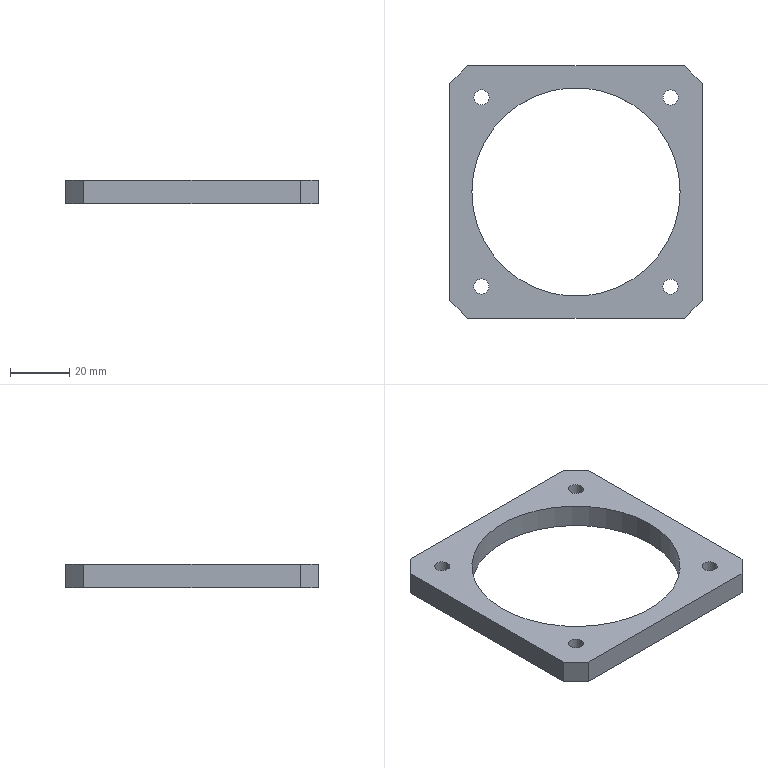NC program | NX | posted with a generic post | part box 85 x 85 x 8 mm
Lines 599 to 1875 of 1875:
(PLANAR_MILL_3 , TOOL : D10C-25L-35L)
N1124 T02 M6
N1126 G54
N1128 G17 G0 G90 X12.135 Y27.325 S4500 M3
N1130 G43 Z20. H2
N1132 Z3.
N1134 G94 G1 X11.608 Y27.587 Z2.995 F1500.
N1136 X8.07 Y28.822 Z2.962
N1138 X4.404 Y29.604 Z2.929
N1140 X0.67 Y29.923 Z2.897
N1142 X-3.075 Y29.772 Z2.864
N1144 X-6.771 Y29.154 Z2.831
N1146 X-10.362 Y28.079 Z2.799
N1148 X-13.79 Y26.564 Z2.766
N1150 X-16.11 Y25.224 Z2.743
N1152 X-19.007 Y23.12 Z2.711
N1154 X-21.632 Y20.685 Z2.68
N1156 X-23.948 Y17.953 Z2.649
N1158 X-25.92 Y14.965 Z2.618
N1160 X-27.522 Y11.763 Z2.586
N1162 X-28.729 Y8.392 Z2.555
N1164 X-29.526 Y4.901 Z2.524
N1166 X-29.9 Y1.34 Z2.493
N1168 Y-1.34 Z2.469
N1170 X-29.526 Y-4.901 Z2.438
N1172 X-28.729 Y-8.392 Z2.407
N1174 X-27.522 Y-11.763 Z2.375
N1176 X-25.92 Y-14.965 Z2.344
N1178 X-23.948 Y-17.953 Z2.313
N1180 X-21.632 Y-20.685 Z2.282
N1182 X-19.007 Y-23.12 Z2.25
N1184 X-16.11 Y-25.224 Z2.219
N1186 X-13.79 Y-26.564 Z2.196
N1188 X-10.362 Y-28.079 Z2.163
N1190 X-6.771 Y-29.154 Z2.13
N1192 X-3.075 Y-29.772 Z2.098
N1194 X0.67 Y-29.923 Z2.065
N1196 X4.404 Y-29.604 Z2.032
N1198 X8.07 Y-28.822 Z2.
N1200 X11.608 Y-27.587 Z1.967
N1202 X14.965 Y-25.92 Z1.934
N1204 X18.087 Y-23.847 Z1.901
N1206 X20.925 Y-21.399 Z1.869
N1208 X23.436 Y-18.616 Z1.836
N1210 X25.579 Y-15.542 Z1.803
N1212 X27.32 Y-12.223 Z1.771
N1214 X28.634 Y-8.713 Z1.738
N1216 X29.498 Y-5.066 Z1.705
N1218 X29.9 Y-1.34 Z1.672
N1220 Y1.34 Z1.649
N1222 X29.498 Y5.066 Z1.616
N1224 X28.634 Y8.713 Z1.584
N1226 X27.32 Y12.223 Z1.551
N1228 X25.579 Y15.542 Z1.518
N1230 X23.436 Y18.616 Z1.486
N1232 X20.925 Y21.399 Z1.453
N1234 X18.087 Y23.847 Z1.42
N1236 X14.965 Y25.92 Z1.387
N1238 X11.608 Y27.587 Z1.355
N1240 X8.07 Y28.822 Z1.322
N1242 X4.404 Y29.604 Z1.289
N1244 X0.67 Y29.923 Z1.257
N1246 X-3.075 Y29.772 Z1.224
N1248 X-6.771 Y29.154 Z1.191
N1250 X-10.362 Y28.079 Z1.159
N1252 X-13.79 Y26.564 Z1.126
N1254 X-16.11 Y25.224 Z1.102
N1256 X-19.007 Y23.12 Z1.071
N1258 X-21.632 Y20.685 Z1.04
N1260 X-23.948 Y17.953 Z1.009
N1262 X-25.92 Y14.965 Z0.977
N1264 X-27.522 Y11.763 Z0.946
N1266 X-28.729 Y8.392 Z0.915
N1268 X-29.526 Y4.901 Z0.884
N1270 X-29.9 Y1.34 Z0.852
N1272 Y-1.34 Z0.829
N1274 X-29.526 Y-4.901 Z0.798
N1276 X-28.729 Y-8.392 Z0.767
N1278 X-27.522 Y-11.763 Z0.735
N1280 X-25.92 Y-14.965 Z0.704
N1282 X-23.948 Y-17.953 Z0.673
N1284 X-21.632 Y-20.685 Z0.642
N1286 X-19.007 Y-23.12 Z0.61
N1288 X-16.11 Y-25.224 Z0.579
N1290 X-13.79 Y-26.564 Z0.556
N1292 X-10.362 Y-28.079 Z0.523
N1294 X-6.771 Y-29.154 Z0.49
N1296 X-3.075 Y-29.772 Z0.458
N1298 X0.67 Y-29.923 Z0.425
N1300 X4.404 Y-29.604 Z0.392
N1302 X8.07 Y-28.822 Z0.359
N1304 X11.608 Y-27.587 Z0.327
N1306 X14.965 Y-25.92 Z0.294
N1308 X18.087 Y-23.847 Z0.261
N1310 X20.925 Y-21.399 Z0.229
N1312 X23.436 Y-18.616 Z0.196
N1314 X25.579 Y-15.542 Z0.163
N1316 X27.32 Y-12.223 Z0.13
N1318 X28.634 Y-8.713 Z0.098
N1320 X29.498 Y-5.066 Z0.065
N1322 X29.9 Y-1.34 Z0.032
N1324 Y1.34 Z0.009
N1326 X29.498 Y5.066 Z-0.024
N1328 X28.634 Y8.713 Z-0.056
N1330 X27.32 Y12.223 Z-0.089
N1332 X25.579 Y15.542 Z-0.122
N1334 X23.436 Y18.616 Z-0.155
N1336 X20.925 Y21.399 Z-0.187
N1338 X18.087 Y23.847 Z-0.22
N1340 X14.965 Y25.92 Z-0.253
N1342 X11.608 Y27.587 Z-0.285
N1344 X8.07 Y28.822 Z-0.318
N1346 X4.404 Y29.604 Z-0.351
N1348 X0.67 Y29.923 Z-0.384
N1350 X-3.075 Y29.772 Z-0.416
N1352 X-6.771 Y29.154 Z-0.449
N1354 X-10.362 Y28.079 Z-0.482
N1356 X-13.79 Y26.564 Z-0.514
N1358 X-16.11 Y25.224 Z-0.538
N1360 X-19.007 Y23.12 Z-0.569
N1362 X-21.632 Y20.685 Z-0.6
N1364 X-23.948 Y17.953 Z-0.631
N1366 X-25.92 Y14.965 Z-0.663
N1368 X-27.522 Y11.763 Z-0.694
N1370 X-28.729 Y8.392 Z-0.725
N1372 X-29.526 Y4.901 Z-0.756
N1374 X-29.9 Y1.34 Z-0.788
N1376 Y-1.34 Z-0.811
N1378 X-29.526 Y-4.901 Z-0.842
N1380 X-28.729 Y-8.392 Z-0.874
N1382 X-27.522 Y-11.763 Z-0.905
N1384 X-25.92 Y-14.965 Z-0.936
N1386 X-23.948 Y-17.953 Z-0.967
N1388 X-21.632 Y-20.685 Z-0.999
N1390 X-19.007 Y-23.12 Z-1.03
N1392 X-16.11 Y-25.224 Z-1.061
N1394 X-13.79 Y-26.564 Z-1.084
N1396 X-10.362 Y-28.079 Z-1.117
N1398 X-6.771 Y-29.154 Z-1.15
N1400 X-3.075 Y-29.772 Z-1.183
N1402 X0.67 Y-29.923 Z-1.215
N1404 X4.404 Y-29.604 Z-1.248
N1406 X8.07 Y-28.822 Z-1.281
N1408 X11.608 Y-27.587 Z-1.313
N1410 X14.965 Y-25.92 Z-1.346
N1412 X18.087 Y-23.847 Z-1.379
N1414 X20.925 Y-21.399 Z-1.412
N1416 X23.436 Y-18.616 Z-1.444
N1418 X25.579 Y-15.542 Z-1.477
N1420 X27.32 Y-12.223 Z-1.51
N1422 X28.634 Y-8.713 Z-1.542
N1424 X29.498 Y-5.066 Z-1.575
N1426 X29.9 Y-1.34 Z-1.608
N1428 Y1.34 Z-1.631
N1430 X29.498 Y5.066 Z-1.664
N1432 X28.634 Y8.713 Z-1.697
N1434 X27.32 Y12.223 Z-1.729
N1436 X25.579 Y15.542 Z-1.762
N1438 X23.436 Y18.616 Z-1.795
N1440 X20.925 Y21.399 Z-1.827
N1442 X18.087 Y23.847 Z-1.86
N1444 X14.965 Y25.92 Z-1.893
N1446 X11.608 Y27.587 Z-1.926
N1448 X8.07 Y28.822 Z-1.958
N1450 X4.404 Y29.604 Z-1.991
N1452 X0.67 Y29.923 Z-2.024
N1454 X-3.075 Y29.772 Z-2.056
N1456 X-6.771 Y29.154 Z-2.089
N1458 X-10.362 Y28.079 Z-2.122
N1460 X-13.79 Y26.564 Z-2.154
N1462 X-16.11 Y25.224 Z-2.178
N1464 X-19.007 Y23.12 Z-2.209
N1466 X-21.632 Y20.685 Z-2.24
N1468 X-23.948 Y17.953 Z-2.272
N1470 X-25.92 Y14.965 Z-2.303
N1472 X-27.522 Y11.763 Z-2.334
N1474 X-28.729 Y8.392 Z-2.365
N1476 X-29.526 Y4.901 Z-2.397
N1478 X-29.9 Y1.34 Z-2.428
N1480 Y-1.34 Z-2.451
N1482 X-29.526 Y-4.901 Z-2.482
N1484 X-28.729 Y-8.392 Z-2.514
N1486 X-27.522 Y-11.763 Z-2.545
N1488 X-25.92 Y-14.965 Z-2.576
N1490 X-23.948 Y-17.953 Z-2.607
N1492 X-21.632 Y-20.685 Z-2.639
N1494 X-19.007 Y-23.12 Z-2.67
N1496 X-16.11 Y-25.224 Z-2.701
N1498 X-13.79 Y-26.564 Z-2.725
N1500 X-10.362 Y-28.079 Z-2.757
N1502 X-6.771 Y-29.154 Z-2.79
N1504 X-3.075 Y-29.772 Z-2.823
N1506 X0.67 Y-29.923 Z-2.855
N1508 X4.404 Y-29.604 Z-2.888
N1510 X8.07 Y-28.822 Z-2.921
N1512 X11.608 Y-27.587 Z-2.954
N1514 X14.965 Y-25.92 Z-2.986
N1516 X18.087 Y-23.847 Z-3.019
N1518 X20.925 Y-21.399 Z-3.052
N1520 X23.436 Y-18.616 Z-3.084
N1522 X25.579 Y-15.542 Z-3.117
N1524 X27.32 Y-12.223 Z-3.15
N1526 X28.634 Y-8.713 Z-3.182
N1528 X29.498 Y-5.066 Z-3.215
N1530 X29.9 Y-1.34 Z-3.248
N1532 Y1.34 Z-3.271
N1534 X29.498 Y5.066 Z-3.304
N1536 X28.634 Y8.713 Z-3.337
N1538 X27.32 Y12.223 Z-3.369
N1540 X25.579 Y15.542 Z-3.402
N1542 X23.436 Y18.616 Z-3.435
N1544 X20.925 Y21.399 Z-3.468
N1546 X18.087 Y23.847 Z-3.5
N1548 X14.965 Y25.92 Z-3.533
N1550 X11.608 Y27.587 Z-3.566
N1552 X8.07 Y28.822 Z-3.598
N1554 X4.404 Y29.604 Z-3.631
N1556 X0.67 Y29.923 Z-3.664
N1558 X-3.075 Y29.772 Z-3.696
N1560 X-6.771 Y29.154 Z-3.729
N1562 X-10.362 Y28.079 Z-3.762
N1564 X-13.79 Y26.564 Z-3.795
N1566 X-16.11 Y25.224 Z-3.818
N1568 X-19.007 Y23.12 Z-3.849
N1570 X-21.632 Y20.685 Z-3.88
N1572 X-23.948 Y17.953 Z-3.912
N1574 X-25.92 Y14.965 Z-3.943
N1576 X-27.522 Y11.763 Z-3.974
N1578 X-28.729 Y8.392 Z-4.005
N1580 X-29.526 Y4.901 Z-4.037
N1582 X-29.9 Y1.34 Z-4.068
N1584 Y-1.34 Z-4.091
N1586 X-29.526 Y-4.901 Z-4.123
N1588 X-28.729 Y-8.392 Z-4.154
N1590 X-27.522 Y-11.763 Z-4.185
N1592 X-25.92 Y-14.965 Z-4.216
N1594 X-23.948 Y-17.953 Z-4.248
N1596 X-21.632 Y-20.685 Z-4.279
N1598 X-19.007 Y-23.12 Z-4.31
N1600 X-16.11 Y-25.224 Z-4.341
N1602 X-13.79 Y-26.564 Z-4.365
N1604 X-10.362 Y-28.079 Z-4.397
N1606 X-6.771 Y-29.154 Z-4.43
N1608 X-3.075 Y-29.772 Z-4.463
N1610 X0.67 Y-29.923 Z-4.496
N1612 X4.404 Y-29.604 Z-4.528
N1614 X8.07 Y-28.822 Z-4.561
N1616 X11.608 Y-27.587 Z-4.594
N1618 X14.965 Y-25.92 Z-4.626
N1620 X18.087 Y-23.847 Z-4.659
N1622 X20.925 Y-21.399 Z-4.692
N1624 X23.436 Y-18.616 Z-4.724
N1626 X25.579 Y-15.542 Z-4.757
N1628 X27.32 Y-12.223 Z-4.79
N1630 X28.634 Y-8.713 Z-4.823
N1632 X29.498 Y-5.066 Z-4.855
N1634 X29.9 Y-1.34 Z-4.888
N1636 Y1.34 Z-4.911
N1638 X29.498 Y5.066 Z-4.944
N1640 X28.634 Y8.713 Z-4.977
N1642 X27.32 Y12.223 Z-5.01
N1644 X25.579 Y15.542 Z-5.042
N1646 X23.436 Y18.616 Z-5.075
N1648 X20.925 Y21.399 Z-5.108
N1650 X18.087 Y23.847 Z-5.14
N1652 X14.965 Y25.92 Z-5.173
N1654 X11.608 Y27.587 Z-5.206
N1656 X8.07 Y28.822 Z-5.238
N1658 X4.404 Y29.604 Z-5.271
N1660 X0.67 Y29.923 Z-5.304
N1662 X-3.075 Y29.772 Z-5.337
N1664 X-6.771 Y29.154 Z-5.369
N1666 X-10.362 Y28.079 Z-5.402
N1668 X-13.79 Y26.564 Z-5.435
N1670 X-16.11 Y25.224 Z-5.458
N1672 X-19.007 Y23.12 Z-5.489
N1674 X-21.632 Y20.685 Z-5.521
N1676 X-23.948 Y17.953 Z-5.552
N1678 X-25.92 Y14.965 Z-5.583
N1680 X-27.522 Y11.763 Z-5.614
N1682 X-28.729 Y8.392 Z-5.646
N1684 X-29.526 Y4.901 Z-5.677
N1686 X-29.9 Y1.34 Z-5.708
N1688 Y-1.34 Z-5.731
N1690 X-29.526 Y-4.901 Z-5.763
N1692 X-28.729 Y-8.392 Z-5.794
N1694 X-27.522 Y-11.763 Z-5.825
N1696 X-25.92 Y-14.965 Z-5.856
N1698 X-23.948 Y-17.953 Z-5.888
N1700 X-21.632 Y-20.685 Z-5.919
N1702 X-19.007 Y-23.12 Z-5.95
N1704 X-16.11 Y-25.224 Z-5.981
N1706 X-13.79 Y-26.564 Z-6.005
N1708 X-10.362 Y-28.079 Z-6.038
N1710 X-6.771 Y-29.154 Z-6.07
N1712 X-3.075 Y-29.772 Z-6.103
N1714 X0.67 Y-29.923 Z-6.136
N1716 X4.404 Y-29.604 Z-6.168
N1718 X8.07 Y-28.822 Z-6.201
N1720 X11.608 Y-27.587 Z-6.234
N1722 X14.965 Y-25.92 Z-6.266
N1724 X18.087 Y-23.847 Z-6.299
N1726 X20.925 Y-21.399 Z-6.332
N1728 X23.436 Y-18.616 Z-6.365
N1730 X25.579 Y-15.542 Z-6.397
N1732 X27.32 Y-12.223 Z-6.43
N1734 X28.634 Y-8.713 Z-6.463
N1736 X29.498 Y-5.066 Z-6.495
N1738 X29.9 Y-1.34 Z-6.528
N1740 Y1.34 Z-6.552
N1742 X29.498 Y5.066 Z-6.584
N1744 X28.634 Y8.713 Z-6.617
N1746 X27.32 Y12.223 Z-6.65
N1748 X25.579 Y15.542 Z-6.682
N1750 X23.436 Y18.616 Z-6.715
N1752 X20.925 Y21.399 Z-6.748
N1754 X18.087 Y23.847 Z-6.78
N1756 X14.965 Y25.92 Z-6.813
N1758 X11.608 Y27.587 Z-6.846
N1760 X8.07 Y28.822 Z-6.879
N1762 X4.404 Y29.604 Z-6.911
N1764 X0.67 Y29.923 Z-6.944
N1766 X-3.075 Y29.772 Z-6.977
N1768 X-6.771 Y29.154 Z-7.009
N1770 X-10.362 Y28.079 Z-7.042
N1772 X-13.79 Y26.564 Z-7.075
N1774 X-16.11 Y25.224 Z-7.098
N1776 X-19.007 Y23.12 Z-7.129
N1778 X-21.632 Y20.685 Z-7.161
N1780 X-23.948 Y17.953 Z-7.192
N1782 X-25.92 Y14.965 Z-7.223
N1784 X-27.522 Y11.763 Z-7.254
N1786 X-28.729 Y8.392 Z-7.286
N1788 X-29.526 Y4.901 Z-7.317
N1790 X-29.9 Y1.34 Z-7.348
N1792 Y-1.34 Z-7.372
N1794 X-29.526 Y-4.901 Z-7.403
N1796 X-28.729 Y-8.392 Z-7.434
N1798 X-27.522 Y-11.763 Z-7.465
N1800 X-25.92 Y-14.965 Z-7.497
N1802 X-23.948 Y-17.953 Z-7.528
N1804 X-21.632 Y-20.685 Z-7.559
N1806 X-19.007 Y-23.12 Z-7.59
N1808 X-16.11 Y-25.224 Z-7.622
N1810 X-13.79 Y-26.564 Z-7.645
N1812 X-10.362 Y-28.079 Z-7.678
N1814 X-6.771 Y-29.154 Z-7.71
N1816 X-3.075 Y-29.772 Z-7.743
N1818 X0.67 Y-29.923 Z-7.776
N1820 X4.404 Y-29.604 Z-7.808
N1822 X8.07 Y-28.822 Z-7.841
N1824 X11.608 Y-27.587 Z-7.874
N1826 X14.965 Y-25.92 Z-7.907
N1828 X18.087 Y-23.847 Z-7.939
N1830 X20.925 Y-21.399 Z-7.972
N1832 X23.436 Y-18.616 Z-8.005
N1834 X25.579 Y-15.542 Z-8.037
N1836 X27.32 Y-12.223 Z-8.07
N1838 X28.634 Y-8.713 Z-8.103
N1840 X29.498 Y-5.066 Z-8.136
N1842 X29.9 Y-1.34 Z-8.168
N1844 Y1.34 Z-8.192
N1846 X29.498 Y5.066 Z-8.224
N1848 X28.634 Y8.713 Z-8.257
N1850 X27.32 Y12.223 Z-8.29
N1852 X25.579 Y15.542 Z-8.322
N1854 X23.436 Y18.616 Z-8.355
N1856 X20.925 Y21.399 Z-8.388
N1858 X18.087 Y23.847 Z-8.421
N1860 X14.965 Y25.92 Z-8.453
N1862 X11.608 Y27.587 Z-8.486
N1864 X8.07 Y28.822 Z-8.519
N1866 X4.404 Y29.604 Z-8.551
N1868 X0.67 Y29.923 Z-8.584
N1870 X-3.075 Y29.772 Z-8.617
N1872 X-6.771 Y29.154 Z-8.65
N1874 X-10.362 Y28.079 Z-8.682
N1876 X-13.79 Y26.564 Z-8.715
N1878 X-16.11 Y25.224 Z-8.738
N1880 X-19.007 Y23.12 Z-8.77
N1882 X-21.632 Y20.685 Z-8.801
N1884 X-23.948 Y17.953 Z-8.832
N1886 X-25.92 Y14.965 Z-8.863
N1888 X-27.522 Y11.763 Z-8.895
N1890 X-28.729 Y8.392 Z-8.926
N1892 X-29.526 Y4.901 Z-8.957
N1894 X-29.9 Y1.34 Z-8.988
N1896 Y0. Z-9.
N1898 G3 X0. Y-29.9 R29.9
N1900 X-29.9 Y0. R-29.9
N1902 G1 Z-6.
N1904 G0 Z20.
(PLANAR_MILL_3_COPY_1 , TOOL : D10C-25L-35L)
N1906 X-5.416 Y-24.318
N1908 Z3.
N1910 G1 X-5.157 Y-24.391 Z2.998
N1912 X-1.875 Y-24.859 Z2.969
N1914 X1.44 Y-24.888 Z2.94
N1916 X4.73 Y-24.477 Z2.911
N1918 X7.936 Y-23.633 Z2.882
N1920 X11.002 Y-22.371 Z2.853
N1922 X13.873 Y-20.713 Z2.824
N1924 X16.499 Y-18.689 Z2.795
N1926 X18.833 Y-16.335 Z2.766
N1928 X20.834 Y-13.691 Z2.737
N1930 X22.466 Y-10.806 Z2.708
N1932 X23.702 Y-7.729 Z2.679
N1934 X24.518 Y-4.516 Z2.65
N1936 X24.9 Y-1.223 Z2.622
N1938 Y1.223 Z2.6
N1940 X24.518 Y4.516 Z2.571
N1942 X23.702 Y7.729 Z2.542
N1944 X22.466 Y10.806 Z2.513
N1946 X20.834 Y13.691 Z2.484
N1948 X18.833 Y16.335 Z2.456
N1950 X16.499 Y18.689 Z2.427
N1952 X13.873 Y20.713 Z2.398
N1954 X11.002 Y22.371 Z2.369
N1956 X7.936 Y23.633 Z2.34
N1958 X4.73 Y24.477 Z2.311
N1960 X1.44 Y24.888 Z2.282
N1962 X-1.875 Y24.859 Z2.253
N1964 X-5.157 Y24.391 Z2.224
N1966 X-8.348 Y23.491 Z2.195
N1968 X-11.391 Y22.175 Z2.166
N1970 X-13.509 Y20.953 Z2.145
N1972 X-16.217 Y18.934 Z2.115
N1974 X-18.627 Y16.569 Z2.086
N1976 X-20.696 Y13.899 Z2.056
N1978 X-22.385 Y10.974 Z2.027
N1980 X-23.663 Y7.848 Z1.997
N1982 X-24.506 Y4.577 Z1.968
N1984 X-24.9 Y1.223 Z1.939
N1986 Y-1.223 Z1.917
N1988 X-24.506 Y-4.577 Z1.888
N1990 X-23.663 Y-7.848 Z1.858
N1992 X-22.385 Y-10.974 Z1.829
N1994 X-20.696 Y-13.899 Z1.799
N1996 X-18.627 Y-16.569 Z1.77
N1998 X-16.217 Y-18.934 Z1.74
N2000 X-13.509 Y-20.953 Z1.711
N2002 X-11.391 Y-22.175 Z1.69
N2004 X-8.348 Y-23.491 Z1.661
N2006 X-5.157 Y-24.391 Z1.632
N2008 X-1.875 Y-24.859 Z1.603
N2010 X1.44 Y-24.888 Z1.574
N2012 X4.73 Y-24.477 Z1.545
N2014 X7.936 Y-23.633 Z1.516
N2016 X11.002 Y-22.371 Z1.487
N2018 X13.873 Y-20.713 Z1.458
N2020 X16.499 Y-18.689 Z1.429
N2022 X18.833 Y-16.335 Z1.4
N2024 X20.834 Y-13.691 Z1.371
N2026 X22.466 Y-10.806 Z1.342
N2028 X23.702 Y-7.729 Z1.313
N2030 X24.518 Y-4.516 Z1.284
N2032 X24.9 Y-1.223 Z1.256
N2034 Y1.223 Z1.234
N2036 X24.518 Y4.516 Z1.205
N2038 X23.702 Y7.729 Z1.176
N2040 X22.466 Y10.806 Z1.147
N2042 X20.834 Y13.691 Z1.118
N2044 X18.833 Y16.335 Z1.09
N2046 X16.499 Y18.689 Z1.061
N2048 X13.873 Y20.713 Z1.032
N2050 X11.002 Y22.371 Z1.003
N2052 X7.936 Y23.633 Z0.974
N2054 X4.73 Y24.477 Z0.945
N2056 X1.44 Y24.888 Z0.916
N2058 X-1.875 Y24.859 Z0.887
N2060 X-5.157 Y24.391 Z0.858
N2062 X-8.348 Y23.491 Z0.829
N2064 X-11.391 Y22.175 Z0.8
N2066 X-13.509 Y20.953 Z0.779
N2068 X-16.217 Y18.934 Z0.749
N2070 X-18.627 Y16.569 Z0.72
N2072 X-20.696 Y13.899 Z0.69
N2074 X-22.385 Y10.974 Z0.661
N2076 X-23.663 Y7.848 Z0.632
N2078 X-24.506 Y4.577 Z0.602
N2080 X-24.9 Y1.223 Z0.573
N2082 Y-1.223 Z0.551
N2084 X-24.506 Y-4.577 Z0.522
N2086 X-23.663 Y-7.848 Z0.492
N2088 X-22.385 Y-10.974 Z0.463
N2090 X-20.696 Y-13.899 Z0.433
N2092 X-18.627 Y-16.569 Z0.404
N2094 X-16.217 Y-18.934 Z0.374
N2096 X-13.509 Y-20.953 Z0.345
N2098 X-11.391 Y-22.175 Z0.324
N2100 X-8.348 Y-23.491 Z0.295
N2102 X-5.157 Y-24.391 Z0.266
N2104 X-1.875 Y-24.859 Z0.237
N2106 X1.44 Y-24.888 Z0.208
N2108 X4.73 Y-24.477 Z0.179
N2110 X7.936 Y-23.633 Z0.15
N2112 X11.002 Y-22.371 Z0.121
N2114 X13.873 Y-20.713 Z0.092
N2116 X16.499 Y-18.689 Z0.063
N2118 X18.833 Y-16.335 Z0.034
N2120 X20.834 Y-13.691 Z0.005
N2122 X22.466 Y-10.806 Z-0.024
N2124 X23.702 Y-7.729 Z-0.053
N2126 X24.518 Y-4.516 Z-0.082
N2128 X24.9 Y-1.223 Z-0.11
N2130 Y1.223 Z-0.132
N2132 X24.518 Y4.516 Z-0.161
N2134 X23.702 Y7.729 Z-0.19
N2136 X22.466 Y10.806 Z-0.219
N2138 X20.834 Y13.691 Z-0.248
N2140 X18.833 Y16.335 Z-0.276
N2142 X16.499 Y18.689 Z-0.305
N2144 X13.873 Y20.713 Z-0.334
N2146 X11.002 Y22.371 Z-0.363
N2148 X7.936 Y23.633 Z-0.392
N2150 X4.73 Y24.477 Z-0.421
N2152 X1.44 Y24.888 Z-0.45
N2154 X-1.875 Y24.859 Z-0.479
N2156 X-5.157 Y24.391 Z-0.508
N2158 X-8.348 Y23.491 Z-0.537
N2160 X-11.391 Y22.175 Z-0.566
N2162 X-13.509 Y20.953 Z-0.587
N2164 X-16.217 Y18.934 Z-0.617
N2166 X-18.627 Y16.569 Z-0.646
N2168 X-20.696 Y13.899 Z-0.676
N2170 X-22.385 Y10.974 Z-0.705
N2172 X-23.663 Y7.848 Z-0.734
N2174 X-24.506 Y4.577 Z-0.764
N2176 X-24.9 Y1.223 Z-0.793
N2178 Y-1.223 Z-0.815
N2180 X-24.506 Y-4.577 Z-0.844
N2182 X-23.663 Y-7.848 Z-0.874
N2184 X-22.385 Y-10.974 Z-0.903
N2186 X-20.696 Y-13.899 Z-0.933
N2188 X-18.627 Y-16.569 Z-0.962
N2190 X-16.217 Y-18.934 Z-0.992
N2192 X-13.509 Y-20.953 Z-1.021
N2194 X-11.391 Y-22.175 Z-1.042
N2196 X-8.348 Y-23.491 Z-1.071
N2198 X-5.157 Y-24.391 Z-1.1
N2200 X-1.875 Y-24.859 Z-1.129
N2202 X1.44 Y-24.888 Z-1.158
N2204 X4.73 Y-24.477 Z-1.187
N2206 X7.936 Y-23.633 Z-1.216
N2208 X11.002 Y-22.371 Z-1.245
N2210 X13.873 Y-20.713 Z-1.274
N2212 X16.499 Y-18.689 Z-1.303
N2214 X18.833 Y-16.335 Z-1.332
N2216 X20.834 Y-13.691 Z-1.361
N2218 X22.466 Y-10.806 Z-1.39
N2220 X23.702 Y-7.729 Z-1.419
N2222 X24.518 Y-4.516 Z-1.447
N2224 X24.9 Y-1.223 Z-1.476
N2226 Y1.223 Z-1.498
N2228 X24.518 Y4.516 Z-1.527
N2230 X23.702 Y7.729 Z-1.556
N2232 X22.466 Y10.806 Z-1.585
N2234 X20.834 Y13.691 Z-1.613
N2236 X18.833 Y16.335 Z-1.642
N2238 X16.499 Y18.689 Z-1.671
N2240 X13.873 Y20.713 Z-1.7
N2242 X11.002 Y22.371 Z-1.729
N2244 X7.936 Y23.633 Z-1.758
N2246 X4.73 Y24.477 Z-1.787
N2248 X1.44 Y24.888 Z-1.816
N2250 X-1.875 Y24.859 Z-1.845
N2252 X-5.157 Y24.391 Z-1.874
N2254 X-8.348 Y23.491 Z-1.903
N2256 X-11.391 Y22.175 Z-1.932
N2258 X-13.509 Y20.953 Z-1.953
N2260 X-16.217 Y18.934 Z-1.983
N2262 X-18.627 Y16.569 Z-2.012
N2264 X-20.696 Y13.899 Z-2.042
N2266 X-22.385 Y10.974 Z-2.071
N2268 X-23.663 Y7.848 Z-2.1
N2270 X-24.506 Y4.577 Z-2.13
N2272 X-24.9 Y1.223 Z-2.159
N2274 Y-1.223 Z-2.181
N2276 X-24.506 Y-4.577 Z-2.21
N2278 X-23.663 Y-7.848 Z-2.24
N2280 X-22.385 Y-10.974 Z-2.269
N2282 X-20.696 Y-13.899 Z-2.299
N2284 X-18.627 Y-16.569 Z-2.328
N2286 X-16.217 Y-18.934 Z-2.358
N2288 X-13.509 Y-20.953 Z-2.387
N2290 X-11.391 Y-22.175 Z-2.408
N2292 X-8.348 Y-23.491 Z-2.437
N2294 X-5.157 Y-24.391 Z-2.466
N2296 X-1.875 Y-24.859 Z-2.495
N2298 X1.44 Y-24.888 Z-2.524
N2300 X4.73 Y-24.477 Z-2.553
N2302 X7.936 Y-23.633 Z-2.582
N2304 X11.002 Y-22.371 Z-2.611
N2306 X13.873 Y-20.713 Z-2.64
N2308 X16.499 Y-18.689 Z-2.669
N2310 X18.833 Y-16.335 Z-2.698
N2312 X20.834 Y-13.691 Z-2.727
N2314 X22.466 Y-10.806 Z-2.756
N2316 X23.702 Y-7.729 Z-2.785
N2318 X24.518 Y-4.516 Z-2.813
N2320 X24.9 Y-1.223 Z-2.842
N2322 Y1.223 Z-2.864
N2324 X24.518 Y4.516 Z-2.893
N2326 X23.702 Y7.729 Z-2.922
N2328 X22.466 Y10.806 Z-2.951
N2330 X20.834 Y13.691 Z-2.979
N2332 X18.833 Y16.335 Z-3.008
N2334 X16.499 Y18.689 Z-3.037
N2336 X13.873 Y20.713 Z-3.066
N2338 X11.002 Y22.371 Z-3.095
N2340 X7.936 Y23.633 Z-3.124
N2342 X4.73 Y24.477 Z-3.153
N2344 X1.44 Y24.888 Z-3.182
N2346 X-1.875 Y24.859 Z-3.211
N2348 X-5.157 Y24.391 Z-3.24
N2350 X-8.348 Y23.491 Z-3.269
N2352 X-11.391 Y22.175 Z-3.298
N2354 X-13.509 Y20.953 Z-3.319
N2356 X-16.217 Y18.934 Z-3.349
N2358 X-18.627 Y16.569 Z-3.378
N2360 X-20.696 Y13.899 Z-3.407
N2362 X-22.385 Y10.974 Z-3.437
N2364 X-23.663 Y7.848 Z-3.466
N2366 X-24.506 Y4.577 Z-3.496
N2368 X-24.9 Y1.223 Z-3.525
N2370 Y-1.223 Z-3.547
N2372 X-24.506 Y-4.577 Z-3.576
N2374 X-23.663 Y-7.848 Z-3.606
N2376 X-22.385 Y-10.974 Z-3.635
N2378 X-20.696 Y-13.899 Z-3.665
N2380 X-18.627 Y-16.569 Z-3.694
N2382 X-16.217 Y-18.934 Z-3.724
N2384 X-13.509 Y-20.953 Z-3.753
N2386 X-11.391 Y-22.175 Z-3.774
N2388 X-8.348 Y-23.491 Z-3.803
N2390 X-5.157 Y-24.391 Z-3.832
N2392 X-1.875 Y-24.859 Z-3.861
N2394 X1.44 Y-24.888 Z-3.89
N2396 X4.73 Y-24.477 Z-3.919
N2398 X7.936 Y-23.633 Z-3.948
N2400 X11.002 Y-22.371 Z-3.977
N2402 X13.873 Y-20.713 Z-4.006
N2404 X16.499 Y-18.689 Z-4.035
N2406 X18.833 Y-16.335 Z-4.064
N2408 X20.834 Y-13.691 Z-4.093
N2410 X22.466 Y-10.806 Z-4.122
N2412 X23.702 Y-7.729 Z-4.151
N2414 X24.518 Y-4.516 Z-4.179
N2416 X24.9 Y-1.223 Z-4.208
N2418 Y1.223 Z-4.23
N2420 X24.518 Y4.516 Z-4.259
N2422 X23.702 Y7.729 Z-4.288
N2424 X22.466 Y10.806 Z-4.317
N2426 X20.834 Y13.691 Z-4.345
N2428 X18.833 Y16.335 Z-4.374
N2430 X16.499 Y18.689 Z-4.403
N2432 X13.873 Y20.713 Z-4.432
N2434 X11.002 Y22.371 Z-4.461
N2436 X7.936 Y23.633 Z-4.49
N2438 X4.73 Y24.477 Z-4.519
N2440 X1.44 Y24.888 Z-4.548
N2442 X-1.875 Y24.859 Z-4.577
N2444 X-5.157 Y24.391 Z-4.606
N2446 X-8.348 Y23.491 Z-4.635
N2448 X-11.391 Y22.175 Z-4.664
N2450 X-13.509 Y20.953 Z-4.685
N2452 X-16.217 Y18.934 Z-4.715
N2454 X-18.627 Y16.569 Z-4.744
N2456 X-20.696 Y13.899 Z-4.773
N2458 X-22.385 Y10.974 Z-4.803
N2460 X-23.663 Y7.848 Z-4.832
N2462 X-24.506 Y4.577 Z-4.862
N2464 X-24.9 Y1.223 Z-4.891
N2466 Y-1.223 Z-4.913
N2468 X-24.506 Y-4.577 Z-4.942
N2470 X-23.663 Y-7.848 Z-4.972
N2472 X-22.385 Y-10.974 Z-5.001
N2474 X-20.696 Y-13.899 Z-5.031
N2476 X-18.627 Y-16.569 Z-5.06
N2478 X-16.217 Y-18.934 Z-5.09
N2480 X-13.509 Y-20.953 Z-5.119
N2482 X-11.391 Y-22.175 Z-5.14
N2484 X-8.348 Y-23.491 Z-5.169
N2486 X-5.157 Y-24.391 Z-5.198
N2488 X-1.875 Y-24.859 Z-5.227
N2490 X1.44 Y-24.888 Z-5.256
N2492 X4.73 Y-24.477 Z-5.285
N2494 X7.936 Y-23.633 Z-5.314
N2496 X11.002 Y-22.371 Z-5.343
N2498 X13.873 Y-20.713 Z-5.372
N2500 X16.499 Y-18.689 Z-5.401
N2502 X18.833 Y-16.335 Z-5.43
N2504 X20.834 Y-13.691 Z-5.459
N2506 X22.466 Y-10.806 Z-5.488
N2508 X23.702 Y-7.729 Z-5.517
N2510 X24.518 Y-4.516 Z-5.545
N2512 X24.9 Y-1.223 Z-5.574
N2514 Y1.223 Z-5.596
N2516 X24.518 Y4.516 Z-5.625
N2518 X23.702 Y7.729 Z-5.654
N2520 X22.466 Y10.806 Z-5.683
N2522 X20.834 Y13.691 Z-5.711
N2524 X18.833 Y16.335 Z-5.74
N2526 X16.499 Y18.689 Z-5.769
N2528 X13.873 Y20.713 Z-5.798
N2530 X11.002 Y22.371 Z-5.827
N2532 X7.936 Y23.633 Z-5.856
N2534 X4.73 Y24.477 Z-5.885
N2536 X1.44 Y24.888 Z-5.914
N2538 X-1.875 Y24.859 Z-5.943
N2540 X-5.157 Y24.391 Z-5.972
N2542 X-8.348 Y23.491 Z-6.001
N2544 X-11.391 Y22.175 Z-6.03
N2546 X-13.509 Y20.953 Z-6.051
N2548 X-16.217 Y18.934 Z-6.081
N2550 X-18.627 Y16.569 Z-6.11
N2552 X-20.696 Y13.899 Z-6.139
N2554 X-22.385 Y10.974 Z-6.169
N2556 X-23.663 Y7.848 Z-6.198
N2558 X-24.506 Y4.577 Z-6.228
N2560 X-24.9 Y1.223 Z-6.257
N2562 Y-1.223 Z-6.279
N2564 X-24.506 Y-4.577 Z-6.308
N2566 X-23.663 Y-7.848 Z-6.338
N2568 X-22.385 Y-10.974 Z-6.367
N2570 X-20.696 Y-13.899 Z-6.397
N2572 X-18.627 Y-16.569 Z-6.426
N2574 X-16.217 Y-18.934 Z-6.456
N2576 X-13.509 Y-20.953 Z-6.485
N2578 X-11.391 Y-22.175 Z-6.506
N2580 X-8.348 Y-23.491 Z-6.535
N2582 X-5.157 Y-24.391 Z-6.564
N2584 X-1.875 Y-24.859 Z-6.593
N2586 X1.44 Y-24.888 Z-6.622
N2588 X4.73 Y-24.477 Z-6.651
N2590 X7.936 Y-23.633 Z-6.68
N2592 X11.002 Y-22.371 Z-6.709
N2594 X13.873 Y-20.713 Z-6.738
N2596 X16.499 Y-18.689 Z-6.767
N2598 X18.833 Y-16.335 Z-6.796
N2600 X20.834 Y-13.691 Z-6.825
N2602 X22.466 Y-10.806 Z-6.854
N2604 X23.702 Y-7.729 Z-6.882
N2606 X24.518 Y-4.516 Z-6.911
N2608 X24.9 Y-1.223 Z-6.94
N2610 Y1.223 Z-6.962
N2612 X24.518 Y4.516 Z-6.991
N2614 X23.702 Y7.729 Z-7.02
N2616 X22.466 Y10.806 Z-7.048
N2618 X20.834 Y13.691 Z-7.077
N2620 X18.833 Y16.335 Z-7.106
N2622 X16.499 Y18.689 Z-7.135
N2624 X13.873 Y20.713 Z-7.164
N2626 X11.002 Y22.371 Z-7.193
N2628 X7.936 Y23.633 Z-7.222
N2630 X4.73 Y24.477 Z-7.251
N2632 X1.44 Y24.888 Z-7.28
N2634 X-1.875 Y24.859 Z-7.309
N2636 X-5.157 Y24.391 Z-7.338
N2638 X-8.348 Y23.491 Z-7.367
N2640 X-11.391 Y22.175 Z-7.396
N2642 X-13.509 Y20.953 Z-7.417
N2644 X-16.217 Y18.934 Z-7.446
N2646 X-18.627 Y16.569 Z-7.476
N2648 X-20.696 Y13.899 Z-7.505
N2650 X-22.385 Y10.974 Z-7.535
N2652 X-23.663 Y7.848 Z-7.564
N2654 X-24.506 Y4.577 Z-7.594
N2656 X-24.9 Y1.223 Z-7.623
N2658 Y-1.223 Z-7.645
N2660 X-24.506 Y-4.577 Z-7.674
N2662 X-23.663 Y-7.848 Z-7.704
N2664 X-22.385 Y-10.974 Z-7.733
N2666 X-20.696 Y-13.899 Z-7.763
N2668 X-18.627 Y-16.569 Z-7.792
N2670 X-16.217 Y-18.934 Z-7.822
N2672 X-13.509 Y-20.953 Z-7.851
N2674 X-11.391 Y-22.175 Z-7.872
N2676 X-8.348 Y-23.491 Z-7.901
N2678 X-5.157 Y-24.391 Z-7.93
N2680 X-1.875 Y-24.859 Z-7.959
N2682 X1.44 Y-24.888 Z-7.988
N2684 X4.73 Y-24.477 Z-8.017
N2686 X7.936 Y-23.633 Z-8.046
N2688 X11.002 Y-22.371 Z-8.075
N2690 X13.873 Y-20.713 Z-8.104
N2692 X16.499 Y-18.689 Z-8.133
N2694 X18.833 Y-16.335 Z-8.162
N2696 X20.834 Y-13.691 Z-8.191
N2698 X22.466 Y-10.806 Z-8.22
N2700 X23.702 Y-7.729 Z-8.248
N2702 X24.518 Y-4.516 Z-8.277
N2704 X24.9 Y-1.223 Z-8.306
N2706 Y1.223 Z-8.328
N2708 X24.518 Y4.516 Z-8.357
N2710 X23.702 Y7.729 Z-8.386
N2712 X22.466 Y10.806 Z-8.414
N2714 X20.834 Y13.691 Z-8.443
N2716 X18.833 Y16.335 Z-8.472
N2718 X16.499 Y18.689 Z-8.501
N2720 X13.873 Y20.713 Z-8.53
N2722 X11.002 Y22.371 Z-8.559
N2724 X7.936 Y23.633 Z-8.588
N2726 X4.73 Y24.477 Z-8.617
N2728 X1.44 Y24.888 Z-8.646
N2730 X-1.875 Y24.859 Z-8.675
N2732 X-5.157 Y24.391 Z-8.704
N2734 X-8.348 Y23.491 Z-8.733
N2736 X-11.391 Y22.175 Z-8.762
N2738 X-13.509 Y20.953 Z-8.783
N2740 X-16.217 Y18.934 Z-8.812
N2742 X-18.627 Y16.569 Z-8.842
N2744 X-20.696 Y13.899 Z-8.871
N2746 X-22.385 Y10.974 Z-8.901
N2748 X-23.663 Y7.848 Z-8.93
N2750 X-24.506 Y4.577 Z-8.96
N2752 X-24.9 Y1.223 Z-8.989
N2754 Y0. Z-9.
N2756 G3 X0. Y-24.9 R24.9
N2758 X-24.9 Y0. R-24.9
N2760 G1 Z-6.
N2762 G0 Z20.
N2764 X12.135 Y27.325
N2766 Z3.
N2768 G1 X11.608 Y27.587 Z2.995
N2770 X8.07 Y28.822 Z2.962
N2772 X4.404 Y29.604 Z2.929
N2774 X0.67 Y29.923 Z2.897
N2776 X-3.075 Y29.772 Z2.864
N2778 X-6.771 Y29.154 Z2.831
N2780 X-10.362 Y28.079 Z2.799
N2782 X-13.79 Y26.564 Z2.766
N2784 X-16.11 Y25.224 Z2.743
N2786 X-19.007 Y23.12 Z2.711
N2788 X-21.632 Y20.685 Z2.68
N2790 X-23.948 Y17.953 Z2.649
N2792 X-25.92 Y14.965 Z2.618
N2794 X-27.522 Y11.763 Z2.586
N2796 X-28.729 Y8.392 Z2.555
N2798 X-29.526 Y4.901 Z2.524
N2800 X-29.9 Y1.34 Z2.493
N2802 Y-1.34 Z2.469
N2804 X-29.526 Y-4.901 Z2.438
N2806 X-28.729 Y-8.392 Z2.407
N2808 X-27.522 Y-11.763 Z2.375
N2810 X-25.92 Y-14.965 Z2.344
N2812 X-23.948 Y-17.953 Z2.313
N2814 X-21.632 Y-20.685 Z2.282
N2816 X-19.007 Y-23.12 Z2.25
N2818 X-16.11 Y-25.224 Z2.219
N2820 X-13.79 Y-26.564 Z2.196
N2822 X-10.362 Y-28.079 Z2.163
N2824 X-6.771 Y-29.154 Z2.13
N2826 X-3.075 Y-29.772 Z2.098
N2828 X0.67 Y-29.923 Z2.065
N2830 X4.404 Y-29.604 Z2.032
N2832 X8.07 Y-28.822 Z2.
N2834 X11.608 Y-27.587 Z1.967
N2836 X14.965 Y-25.92 Z1.934
N2838 X18.087 Y-23.847 Z1.901
N2840 X20.925 Y-21.399 Z1.869
N2842 X23.436 Y-18.616 Z1.836
N2844 X25.579 Y-15.542 Z1.803
N2846 X27.32 Y-12.223 Z1.771
N2848 X28.634 Y-8.713 Z1.738
N2850 X29.498 Y-5.066 Z1.705
N2852 X29.9 Y-1.34 Z1.672
N2854 Y1.34 Z1.649
N2856 X29.498 Y5.066 Z1.616
N2858 X28.634 Y8.713 Z1.584
N2860 X27.32 Y12.223 Z1.551
N2862 X25.579 Y15.542 Z1.518
N2864 X23.436 Y18.616 Z1.486
N2866 X20.925 Y21.399 Z1.453
N2868 X18.087 Y23.847 Z1.42
N2870 X14.965 Y25.92 Z1.387
N2872 X11.608 Y27.587 Z1.355
N2874 X8.07 Y28.822 Z1.322
N2876 X4.404 Y29.604 Z1.289
N2878 X0.67 Y29.923 Z1.257
N2880 X-3.075 Y29.772 Z1.224
N2882 X-6.771 Y29.154 Z1.191
N2884 X-10.362 Y28.079 Z1.159
N2886 X-13.79 Y26.564 Z1.126
N2888 X-16.11 Y25.224 Z1.102
N2890 X-19.007 Y23.12 Z1.071
N2892 X-21.632 Y20.685 Z1.04
N2894 X-23.948 Y17.953 Z1.009
N2896 X-25.92 Y14.965 Z0.977
N2898 X-27.522 Y11.763 Z0.946
N2900 X-28.729 Y8.392 Z0.915
N2902 X-29.526 Y4.901 Z0.884
N2904 X-29.9 Y1.34 Z0.852
N2906 Y-1.34 Z0.829
N2908 X-29.526 Y-4.901 Z0.798
N2910 X-28.729 Y-8.392 Z0.767
N2912 X-27.522 Y-11.763 Z0.735
N2914 X-25.92 Y-14.965 Z0.704
N2916 X-23.948 Y-17.953 Z0.673
N2918 X-21.632 Y-20.685 Z0.642
N2920 X-19.007 Y-23.12 Z0.61
N2922 X-16.11 Y-25.224 Z0.579
N2924 X-13.79 Y-26.564 Z0.556
N2926 X-10.362 Y-28.079 Z0.523
N2928 X-6.771 Y-29.154 Z0.49
N2930 X-3.075 Y-29.772 Z0.458
N2932 X0.67 Y-29.923 Z0.425
N2934 X4.404 Y-29.604 Z0.392
N2936 X8.07 Y-28.822 Z0.359
N2938 X11.608 Y-27.587 Z0.327
N2940 X14.965 Y-25.92 Z0.294
N2942 X18.087 Y-23.847 Z0.261
N2944 X20.925 Y-21.399 Z0.229
N2946 X23.436 Y-18.616 Z0.196
N2948 X25.579 Y-15.542 Z0.163
N2950 X27.32 Y-12.223 Z0.13
N2952 X28.634 Y-8.713 Z0.098
N2954 X29.498 Y-5.066 Z0.065
N2956 X29.9 Y-1.34 Z0.032
N2958 Y1.34 Z0.009
N2960 X29.498 Y5.066 Z-0.024
N2962 X28.634 Y8.713 Z-0.056
N2964 X27.32 Y12.223 Z-0.089
N2966 X25.579 Y15.542 Z-0.122
N2968 X23.436 Y18.616 Z-0.155
N2970 X20.925 Y21.399 Z-0.187
N2972 X18.087 Y23.847 Z-0.22
N2974 X14.965 Y25.92 Z-0.253
N2976 X11.608 Y27.587 Z-0.285
N2978 X8.07 Y28.822 Z-0.318
N2980 X4.404 Y29.604 Z-0.351
N2982 X0.67 Y29.923 Z-0.384
N2984 X-3.075 Y29.772 Z-0.416
N2986 X-6.771 Y29.154 Z-0.449
N2988 X-10.362 Y28.079 Z-0.482
N2990 X-13.79 Y26.564 Z-0.514
N2992 X-16.11 Y25.224 Z-0.538
N2994 X-19.007 Y23.12 Z-0.569
N2996 X-21.632 Y20.685 Z-0.6
N2998 X-23.948 Y17.953 Z-0.631
N3000 X-25.92 Y14.965 Z-0.663
N3002 X-27.522 Y11.763 Z-0.694
N3004 X-28.729 Y8.392 Z-0.725
N3006 X-29.526 Y4.901 Z-0.756
N3008 X-29.9 Y1.34 Z-0.788
N3010 Y-1.34 Z-0.811
N3012 X-29.526 Y-4.901 Z-0.842
N3014 X-28.729 Y-8.392 Z-0.874
N3016 X-27.522 Y-11.763 Z-0.905
N3018 X-25.92 Y-14.965 Z-0.936
N3020 X-23.948 Y-17.953 Z-0.967
N3022 X-21.632 Y-20.685 Z-0.999
N3024 X-19.007 Y-23.12 Z-1.03
N3026 X-16.11 Y-25.224 Z-1.061
N3028 X-13.79 Y-26.564 Z-1.084
N3030 X-10.362 Y-28.079 Z-1.117
N3032 X-6.771 Y-29.154 Z-1.15
N3034 X-3.075 Y-29.772 Z-1.183
N3036 X0.67 Y-29.923 Z-1.215
N3038 X4.404 Y-29.604 Z-1.248
N3040 X8.07 Y-28.822 Z-1.281
N3042 X11.608 Y-27.587 Z-1.313
N3044 X14.965 Y-25.92 Z-1.346
N3046 X18.087 Y-23.847 Z-1.379
N3048 X20.925 Y-21.399 Z-1.412
N3050 X23.436 Y-18.616 Z-1.444
N3052 X25.579 Y-15.542 Z-1.477
N3054 X27.32 Y-12.223 Z-1.51
N3056 X28.634 Y-8.713 Z-1.542
N3058 X29.498 Y-5.066 Z-1.575
N3060 X29.9 Y-1.34 Z-1.608
N3062 Y1.34 Z-1.631
N3064 X29.498 Y5.066 Z-1.664
N3066 X28.634 Y8.713 Z-1.697
N3068 X27.32 Y12.223 Z-1.729
N3070 X25.579 Y15.542 Z-1.762
N3072 X23.436 Y18.616 Z-1.795
N3074 X20.925 Y21.399 Z-1.827
N3076 X18.087 Y23.847 Z-1.86
N3078 X14.965 Y25.92 Z-1.893
N3080 X11.608 Y27.587 Z-1.926
N3082 X8.07 Y28.822 Z-1.958
N3084 X4.404 Y29.604 Z-1.991
N3086 X0.67 Y29.923 Z-2.024
N3088 X-3.075 Y29.772 Z-2.056
N3090 X-6.771 Y29.154 Z-2.089
N3092 X-10.362 Y28.079 Z-2.122
N3094 X-13.79 Y26.564 Z-2.154
N3096 X-16.11 Y25.224 Z-2.178
N3098 X-19.007 Y23.12 Z-2.209
N3100 X-21.632 Y20.685 Z-2.24
N3102 X-23.948 Y17.953 Z-2.272
N3104 X-25.92 Y14.965 Z-2.303
N3106 X-27.522 Y11.763 Z-2.334
N3108 X-28.729 Y8.392 Z-2.365
N3110 X-29.526 Y4.901 Z-2.397
N3112 X-29.9 Y1.34 Z-2.428
N3114 Y-1.34 Z-2.451
N3116 X-29.526 Y-4.901 Z-2.482
N3118 X-28.729 Y-8.392 Z-2.514
N3120 X-27.522 Y-11.763 Z-2.545
N3122 X-25.92 Y-14.965 Z-2.576
N3124 X-23.948 Y-17.953 Z-2.607
N3126 X-21.632 Y-20.685 Z-2.639
N3128 X-19.007 Y-23.12 Z-2.67
N3130 X-16.11 Y-25.224 Z-2.701
N3132 X-13.79 Y-26.564 Z-2.725
N3134 X-10.362 Y-28.079 Z-2.757
N3136 X-6.771 Y-29.154 Z-2.79
N3138 X-3.075 Y-29.772 Z-2.823
N3140 X0.67 Y-29.923 Z-2.855
N3142 X4.404 Y-29.604 Z-2.888
N3144 X8.07 Y-28.822 Z-2.921
N3146 X11.608 Y-27.587 Z-2.954
N3148 X14.965 Y-25.92 Z-2.986
N3150 X18.087 Y-23.847 Z-3.019
N3152 X20.925 Y-21.399 Z-3.052
N3154 X23.436 Y-18.616 Z-3.084
N3156 X25.579 Y-15.542 Z-3.117
N3158 X27.32 Y-12.223 Z-3.15
N3160 X28.634 Y-8.713 Z-3.182
N3162 X29.498 Y-5.066 Z-3.215
N3164 X29.9 Y-1.34 Z-3.248
N3166 Y1.34 Z-3.271
N3168 X29.498 Y5.066 Z-3.304
N3170 X28.634 Y8.713 Z-3.337
N3172 X27.32 Y12.223 Z-3.369
N3174 X25.579 Y15.542 Z-3.402
N3176 X23.436 Y18.616 Z-3.435
N3178 X20.925 Y21.399 Z-3.468
N3180 X18.087 Y23.847 Z-3.5
N3182 X14.965 Y25.92 Z-3.533
N3184 X11.608 Y27.587 Z-3.566
N3186 X8.07 Y28.822 Z-3.598
N3188 X4.404 Y29.604 Z-3.631
N3190 X0.67 Y29.923 Z-3.664
N3192 X-3.075 Y29.772 Z-3.696
N3194 X-6.771 Y29.154 Z-3.729
N3196 X-10.362 Y28.079 Z-3.762
N3198 X-13.79 Y26.564 Z-3.795
N3200 X-16.11 Y25.224 Z-3.818
N3202 X-19.007 Y23.12 Z-3.849
N3204 X-21.632 Y20.685 Z-3.88
N3206 X-23.948 Y17.953 Z-3.912
N3208 X-25.92 Y14.965 Z-3.943
N3210 X-27.522 Y11.763 Z-3.974
N3212 X-28.729 Y8.392 Z-4.005
N3214 X-29.526 Y4.901 Z-4.037
N3216 X-29.9 Y1.34 Z-4.068
N3218 Y-1.34 Z-4.091
N3220 X-29.526 Y-4.901 Z-4.123
N3222 X-28.729 Y-8.392 Z-4.154
N3224 X-27.522 Y-11.763 Z-4.185
N3226 X-25.92 Y-14.965 Z-4.216
N3228 X-23.948 Y-17.953 Z-4.248
N3230 X-21.632 Y-20.685 Z-4.279
N3232 X-19.007 Y-23.12 Z-4.31
N3234 X-16.11 Y-25.224 Z-4.341
N3236 X-13.79 Y-26.564 Z-4.365
N3238 X-10.362 Y-28.079 Z-4.397
N3240 X-6.771 Y-29.154 Z-4.43
N3242 X-3.075 Y-29.772 Z-4.463
N3244 X0.67 Y-29.923 Z-4.496
N3246 X4.404 Y-29.604 Z-4.528
N3248 X8.07 Y-28.822 Z-4.561
N3250 X11.608 Y-27.587 Z-4.594
N3252 X14.965 Y-25.92 Z-4.626
N3254 X18.087 Y-23.847 Z-4.659
N3256 X20.925 Y-21.399 Z-4.692
N3258 X23.436 Y-18.616 Z-4.724
N3260 X25.579 Y-15.542 Z-4.757
N3262 X27.32 Y-12.223 Z-4.79
N3264 X28.634 Y-8.713 Z-4.823
N3266 X29.498 Y-5.066 Z-4.855
N3268 X29.9 Y-1.34 Z-4.888
N3270 Y1.34 Z-4.911
N3272 X29.498 Y5.066 Z-4.944
N3274 X28.634 Y8.713 Z-4.977
N3276 X27.32 Y12.223 Z-5.01
N3278 X25.579 Y15.542 Z-5.042
N3280 X23.436 Y18.616 Z-5.075
N3282 X20.925 Y21.399 Z-5.108
N3284 X18.087 Y23.847 Z-5.14
N3286 X14.965 Y25.92 Z-5.173
N3288 X11.608 Y27.587 Z-5.206
N3290 X8.07 Y28.822 Z-5.238
N3292 X4.404 Y29.604 Z-5.271
N3294 X0.67 Y29.923 Z-5.304
N3296 X-3.075 Y29.772 Z-5.337
N3298 X-6.771 Y29.154 Z-5.369
N3300 X-10.362 Y28.079 Z-5.402
N3302 X-13.79 Y26.564 Z-5.435
N3304 X-16.11 Y25.224 Z-5.458
N3306 X-19.007 Y23.12 Z-5.489
N3308 X-21.632 Y20.685 Z-5.521
N3310 X-23.948 Y17.953 Z-5.552
N3312 X-25.92 Y14.965 Z-5.583
N3314 X-27.522 Y11.763 Z-5.614
N3316 X-28.729 Y8.392 Z-5.646
N3318 X-29.526 Y4.901 Z-5.677
N3320 X-29.9 Y1.34 Z-5.708
N3322 Y-1.34 Z-5.731
N3324 X-29.526 Y-4.901 Z-5.763
N3326 X-28.729 Y-8.392 Z-5.794
N3328 X-27.522 Y-11.763 Z-5.825
N3330 X-25.92 Y-14.965 Z-5.856
N3332 X-23.948 Y-17.953 Z-5.888
N3334 X-21.632 Y-20.685 Z-5.919
N3336 X-19.007 Y-23.12 Z-5.95
N3338 X-16.11 Y-25.224 Z-5.981
N3340 X-13.79 Y-26.564 Z-6.005
N3342 X-10.362 Y-28.079 Z-6.038
N3344 X-6.771 Y-29.154 Z-6.07
N3346 X-3.075 Y-29.772 Z-6.103
N3348 X0.67 Y-29.923 Z-6.136
N3350 X4.404 Y-29.604 Z-6.168
N3352 X8.07 Y-28.822 Z-6.201
N3354 X11.608 Y-27.587 Z-6.234
N3356 X14.965 Y-25.92 Z-6.266
N3358 X18.087 Y-23.847 Z-6.299
N3360 X20.925 Y-21.399 Z-6.332
N3362 X23.436 Y-18.616 Z-6.365
N3364 X25.579 Y-15.542 Z-6.397
N3366 X27.32 Y-12.223 Z-6.43
N3368 X28.634 Y-8.713 Z-6.463
N3370 X29.498 Y-5.066 Z-6.495
N3372 X29.9 Y-1.34 Z-6.528
N3374 Y1.34 Z-6.552
N3376 X29.498 Y5.066 Z-6.584
N3378 X28.634 Y8.713 Z-6.617
N3380 X27.32 Y12.223 Z-6.65
N3382 X25.579 Y15.542 Z-6.682
N3384 X23.436 Y18.616 Z-6.715
N3386 X20.925 Y21.399 Z-6.748
N3388 X18.087 Y23.847 Z-6.78
N3390 X14.965 Y25.92 Z-6.813
N3392 X11.608 Y27.587 Z-6.846
N3394 X8.07 Y28.822 Z-6.879
N3396 X4.404 Y29.604 Z-6.911
N3398 X0.67 Y29.923 Z-6.944
N3400 X-3.075 Y29.772 Z-6.977
N3402 X-6.771 Y29.154 Z-7.009
N3404 X-10.362 Y28.079 Z-7.042
N3406 X-13.79 Y26.564 Z-7.075
N3408 X-16.11 Y25.224 Z-7.098
N3410 X-19.007 Y23.12 Z-7.129
N3412 X-21.632 Y20.685 Z-7.161
N3414 X-23.948 Y17.953 Z-7.192
N3416 X-25.92 Y14.965 Z-7.223
N3418 X-27.522 Y11.763 Z-7.254
N3420 X-28.729 Y8.392 Z-7.286
N3422 X-29.526 Y4.901 Z-7.317
N3424 X-29.9 Y1.34 Z-7.348
N3426 Y-1.34 Z-7.372
N3428 X-29.526 Y-4.901 Z-7.403
N3430 X-28.729 Y-8.392 Z-7.434
N3432 X-27.522 Y-11.763 Z-7.465
N3434 X-25.92 Y-14.965 Z-7.497
N3436 X-23.948 Y-17.953 Z-7.528
N3438 X-21.632 Y-20.685 Z-7.559
N3440 X-19.007 Y-23.12 Z-7.59
N3442 X-16.11 Y-25.224 Z-7.622
N3444 X-13.79 Y-26.564 Z-7.645
N3446 X-10.362 Y-28.079 Z-7.678
N3448 X-6.771 Y-29.154 Z-7.71
N3450 X-3.075 Y-29.772 Z-7.743
N3452 X0.67 Y-29.923 Z-7.776
N3454 X4.404 Y-29.604 Z-7.808
N3456 X8.07 Y-28.822 Z-7.841
N3458 X11.608 Y-27.587 Z-7.874
N3460 X14.965 Y-25.92 Z-7.907
N3462 X18.087 Y-23.847 Z-7.939
N3464 X20.925 Y-21.399 Z-7.972
N3466 X23.436 Y-18.616 Z-8.005
N3468 X25.579 Y-15.542 Z-8.037
N3470 X27.32 Y-12.223 Z-8.07
N3472 X28.634 Y-8.713 Z-8.103
N3474 X29.498 Y-5.066 Z-8.136
N3476 X29.9 Y-1.34 Z-8.168
N3478 Y1.34 Z-8.192
N3480 X29.498 Y5.066 Z-8.224
N3482 X28.634 Y8.713 Z-8.257
N3484 X27.32 Y12.223 Z-8.29
N3486 X25.579 Y15.542 Z-8.322
N3488 X23.436 Y18.616 Z-8.355
N3490 X20.925 Y21.399 Z-8.388
N3492 X18.087 Y23.847 Z-8.421
N3494 X14.965 Y25.92 Z-8.453
N3496 X11.608 Y27.587 Z-8.486
N3498 X8.07 Y28.822 Z-8.519
N3500 X4.404 Y29.604 Z-8.551
N3502 X0.67 Y29.923 Z-8.584
N3504 X-3.075 Y29.772 Z-8.617
N3506 X-6.771 Y29.154 Z-8.65
N3508 X-10.362 Y28.079 Z-8.682
N3510 X-13.79 Y26.564 Z-8.715
N3512 X-16.11 Y25.224 Z-8.738
N3514 X-19.007 Y23.12 Z-8.77
N3516 X-21.632 Y20.685 Z-8.801
N3518 X-23.948 Y17.953 Z-8.832
N3520 X-25.92 Y14.965 Z-8.863
N3522 X-27.522 Y11.763 Z-8.895
N3524 X-28.729 Y8.392 Z-8.926
N3526 X-29.526 Y4.901 Z-8.957
N3528 X-29.9 Y1.34 Z-8.988
N3530 Y0. Z-9.
N3532 G3 X0. Y-29.9 R29.9
N3534 X-29.9 Y0. R-29.9
N3536 G1 Z-6.
N3538 G0 Z20.
N3540 M5
(PLANAR_MILL_3_COPY , TOOL : 8J-20L-30L)
N3542 T03 M6
N3544 G54
N3546 G17 G0 G90 X-29.6 Y0.913 S3500 M3
N3548 G43 Z20. H3
N3550 Z-6.
N3552 G94 G1 Z-9. F800.
N3554 G41 X-30.093 Y1. D3
N3556 X-30.109
N3558 G3 X-31.109 Y0. R1.
N3560 X0. Y-31.109 R31.109
N3562 X-31.109 Y0. R-31.109
N3564 X-30.109 Y-1. R1.
N3566 G40
N3568 G1 X-29.617 Y-0.913
N3570 X-29.618 Y0.913
N3572 G41 X-30.11 Y1.
N3574 G3 X-31.11 Y0. R1.
N3576 X0. Y-31.11 R31.11
N3578 X-31.11 Y0. R-31.11
N3580 X-30.11 Y-1. R1.
N3582 G1 X-30.093
N3584 G40
N3586 X-29.601 Y-0.913
N3588 Z-6.
N3590 G0 Z20.
N3592 M5
(PLANAR_MILL_2_COPY_1 , TOOL : D4反刮刀)
N3594 T06 M6
N3596 G54
N3598 G17 G0 G90 X-31.537 Y2. S3500 M3
N3600 G43 Z20. H6
N3602 Z2.5
N3604 G94 G1 Z-0.5 F1000.
N3606 X-31.6
N3608 G3 X-33.6 Y0. R2.
N3610 X0. Y-33.6 R33.6
N3612 X-33.6 Y0. R-33.6
N3614 X-31.6 Y-2. R2.
N3616 G1 X-31.537
N3618 Z2.5
N3620 G0 Z20.
(PLANAR_MILL_2_COPY_COPY , TOOL : D4反刮刀)
N3622 X-31.186 Y2.
N3624 Z-5.95
N3626 G1 Z-8.95
N3628 X-31.25
N3630 G3 X-33.25 Y0. R2.
N3632 X0. Y-33.25 R33.25
N3634 X-33.25 Y0. R-33.25
N3636 X-31.25 Y-2. R2.
N3638 G1 X-31.186
N3640 Z-5.95
N3642 G0 Z20.
N3644 M5
N3646 M2